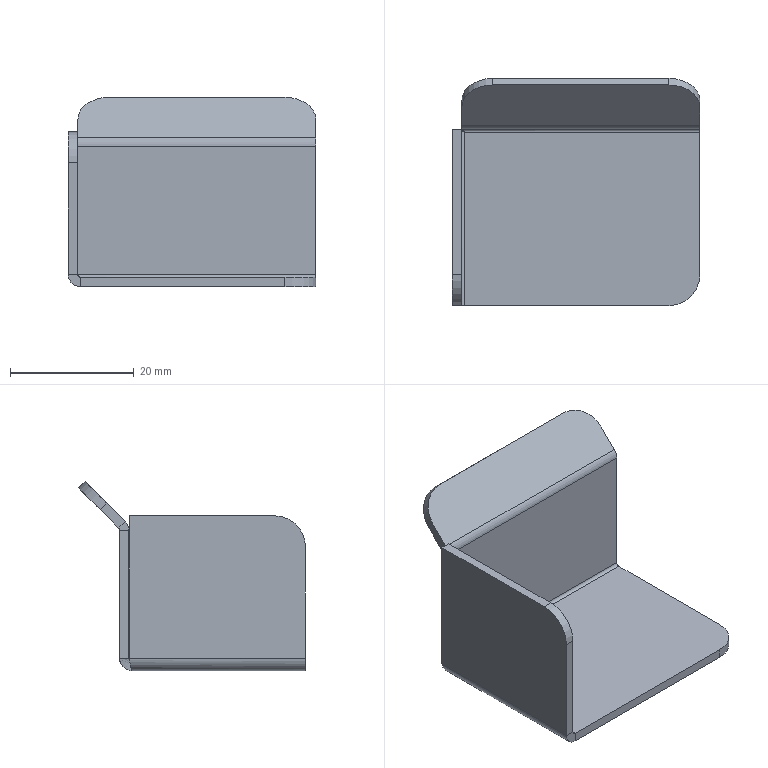Part | SolidWorks | features BaseBody 1 | 1 solid | 34 faces | box 40 x 36.632 x 30.571 mm | volume 4517 mm3 | plane 22 | cylinder 10 | spline 2 | commonest cylinder face diameters 10 x4 1 x3 4 x3
STEP:
#1=CARTESIAN_POINT('',(-13.429,20.571,29.071));
#2=VERTEX_POINT('',#1);
#3=CARTESIAN_POINT('',(-18.429,17.036,25.536));
#4=VERTEX_POINT('',#3);
#5=CARTESIAN_POINT('',(-13.429,17.036,25.536));
#6=DIRECTION('',(0.,-0.7071,0.7071));
#7=DIRECTION('',(0.,0.7071,0.7071));
#8=AXIS2_PLACEMENT_3D('',#5,#6,#7);
#9=CIRCLE('',#8,5.);
#10=EDGE_CURVE('',#2,#4,#9,.T.);
#11=ORIENTED_EDGE('',*,*,#10,.F.);
#12=CARTESIAN_POINT('',(-13.429,21.632,28.01));
#13=VERTEX_POINT('',#12);
#14=CARTESIAN_POINT('',(-13.429,20.571,29.071));
#15=DIRECTION('',(0.,-0.7071,0.7071));
#16=VECTOR('',#15,1000.);
#17=LINE('',#14,#16);
#18=EDGE_CURVE('',#13,#2,#17,.T.);
#19=ORIENTED_EDGE('',*,*,#18,.F.);
#20=CARTESIAN_POINT('',(-18.429,18.096,24.475));
#21=VERTEX_POINT('',#20);
#22=CARTESIAN_POINT('',(-13.429,18.096,24.475));
#23=DIRECTION('',(0.,0.7071,-0.7071));
#24=DIRECTION('',(0.,0.7071,0.7071));
#25=AXIS2_PLACEMENT_3D('',#22,#23,#24);
#26=CIRCLE('',#25,5.);
#27=EDGE_CURVE('',#21,#13,#26,.T.);
#28=ORIENTED_EDGE('',*,*,#27,.F.);
#29=CARTESIAN_POINT('',(-18.429,17.036,25.536));
#30=DIRECTION('',(0.,0.7071,-0.7071));
#31=VECTOR('',#30,1000.);
#32=LINE('',#29,#31);
#33=EDGE_CURVE('',#4,#21,#32,.T.);
#34=ORIENTED_EDGE('',*,*,#33,.F.);
#35=EDGE_LOOP('',(#11,#19,#28,#34));
#36=FACE_OUTER_BOUND('',#35,.T.);
#37=CARTESIAN_POINT('',(-13.429,17.036,25.536));
#38=DIRECTION('',(0.,0.7071,-0.7071));
#39=DIRECTION('',(0.,0.7071,0.7071));
#40=AXIS2_PLACEMENT_3D('',#37,#38,#39);
#41=CYLINDRICAL_SURFACE('',#40,5.);
#42=ADVANCED_FACE('',(#36),#41,.T.);
#43=CARTESIAN_POINT('',(20.,17.036,25.536));
#44=VERTEX_POINT('',#43);
#45=CARTESIAN_POINT('',(15.,20.571,29.071));
#46=VERTEX_POINT('',#45);
#47=CARTESIAN_POINT('',(15.,17.036,25.536));
#48=DIRECTION('',(0.,-0.7071,0.7071));
#49=DIRECTION('',(0.,0.7071,0.7071));
#50=AXIS2_PLACEMENT_3D('',#47,#48,#49);
#51=CIRCLE('',#50,5.);
#52=EDGE_CURVE('',#44,#46,#51,.T.);
#53=ORIENTED_EDGE('',*,*,#52,.F.);
#54=CARTESIAN_POINT('',(20.,18.096,24.475));
#55=VERTEX_POINT('',#54);
#56=CARTESIAN_POINT('',(20.,17.036,25.536));
#57=DIRECTION('',(0.,-0.7071,0.7071));
#58=VECTOR('',#57,1000.);
#59=LINE('',#56,#58);
#60=EDGE_CURVE('',#55,#44,#59,.T.);
#61=ORIENTED_EDGE('',*,*,#60,.F.);
#62=CARTESIAN_POINT('',(15.,21.632,28.01));
#63=VERTEX_POINT('',#62);
#64=CARTESIAN_POINT('',(15.,18.096,24.475));
#65=DIRECTION('',(0.,0.7071,-0.7071));
#66=DIRECTION('',(0.,0.7071,0.7071));
#67=AXIS2_PLACEMENT_3D('',#64,#65,#66);
#68=CIRCLE('',#67,5.);
#69=EDGE_CURVE('',#63,#55,#68,.T.);
#70=ORIENTED_EDGE('',*,*,#69,.F.);
#71=CARTESIAN_POINT('',(15.,20.571,29.071));
#72=DIRECTION('',(0.,0.7071,-0.7071));
#73=VECTOR('',#72,1000.);
#74=LINE('',#71,#73);
#75=EDGE_CURVE('',#46,#63,#74,.T.);
#76=ORIENTED_EDGE('',*,*,#75,.F.);
#77=EDGE_LOOP('',(#53,#61,#70,#76));
#78=FACE_OUTER_BOUND('',#77,.T.);
#79=CARTESIAN_POINT('',(15.,17.036,25.536));
#80=DIRECTION('',(0.,0.7071,-0.7071));
#81=DIRECTION('',(0.,0.7071,0.7071));
#82=AXIS2_PLACEMENT_3D('',#79,#80,#81);
#83=CYLINDRICAL_SURFACE('',#82,5.);
#84=ADVANCED_FACE('',(#78),#83,.T.);
#85=CARTESIAN_POINT('',(-20.,-15.,18.5));
#86=VERTEX_POINT('',#85);
#87=CARTESIAN_POINT('',(-20.,-10.,23.5));
#88=VERTEX_POINT('',#87);
#89=CARTESIAN_POINT('',(-20.,-10.,18.5));
#90=DIRECTION('',(-1.,0.,0.));
#91=DIRECTION('',(0.,0.,-1.));
#92=AXIS2_PLACEMENT_3D('',#89,#90,#91);
#93=CIRCLE('',#92,5.);
#94=EDGE_CURVE('',#86,#88,#93,.T.);
#95=ORIENTED_EDGE('',*,*,#94,.F.);
#96=CARTESIAN_POINT('',(-18.5,-15.,18.5));
#97=VERTEX_POINT('',#96);
#98=CARTESIAN_POINT('',(-20.,-15.,18.5));
#99=DIRECTION('',(-1.,0.,0.));
#100=VECTOR('',#99,1000.);
#101=LINE('',#98,#100);
#102=EDGE_CURVE('',#97,#86,#101,.T.);
#103=ORIENTED_EDGE('',*,*,#102,.F.);
#104=CARTESIAN_POINT('',(-18.5,-10.,23.5));
#105=VERTEX_POINT('',#104);
#106=CARTESIAN_POINT('',(-18.5,-10.,18.5));
#107=DIRECTION('',(1.,0.,0.));
#108=DIRECTION('',(0.,0.,-1.));
#109=AXIS2_PLACEMENT_3D('',#106,#107,#108);
#110=CIRCLE('',#109,5.);
#111=EDGE_CURVE('',#105,#97,#110,.T.);
#112=ORIENTED_EDGE('',*,*,#111,.F.);
#113=CARTESIAN_POINT('',(-20.,-10.,23.5));
#114=DIRECTION('',(1.,0.,0.));
#115=VECTOR('',#114,1000.);
#116=LINE('',#113,#115);
#117=EDGE_CURVE('',#88,#105,#116,.T.);
#118=ORIENTED_EDGE('',*,*,#117,.F.);
#119=EDGE_LOOP('',(#95,#103,#112,#118));
#120=FACE_OUTER_BOUND('',#119,.T.);
#121=CARTESIAN_POINT('',(-20.,-10.,18.5));
#122=DIRECTION('',(1.,0.,0.));
#123=DIRECTION('',(0.,0.,-1.));
#124=AXIS2_PLACEMENT_3D('',#121,#122,#123);
#125=CYLINDRICAL_SURFACE('',#124,5.);
#126=ADVANCED_FACE('',(#120),#125,.T.);
#127=CARTESIAN_POINT('',(20.,-10.,-1.5));
#128=VERTEX_POINT('',#127);
#129=CARTESIAN_POINT('',(15.,-15.,-1.5));
#130=VERTEX_POINT('',#129);
#131=CARTESIAN_POINT('',(15.,-10.,-1.5));
#132=DIRECTION('',(0.,0.,-1.));
#133=DIRECTION('',(-1.,0.,0.));
#134=AXIS2_PLACEMENT_3D('',#131,#132,#133);
#135=CIRCLE('',#134,5.);
#136=EDGE_CURVE('',#128,#130,#135,.T.);
#137=ORIENTED_EDGE('',*,*,#136,.F.);
#138=CARTESIAN_POINT('',(20.,-10.,0.));
#139=VERTEX_POINT('',#138);
#140=CARTESIAN_POINT('',(20.,-10.,-1.5));
#141=DIRECTION('',(0.,0.,-1.));
#142=VECTOR('',#141,1000.);
#143=LINE('',#140,#142);
#144=EDGE_CURVE('',#139,#128,#143,.T.);
#145=ORIENTED_EDGE('',*,*,#144,.F.);
#146=CARTESIAN_POINT('',(15.,-15.,0.));
#147=VERTEX_POINT('',#146);
#148=CARTESIAN_POINT('',(15.,-10.,0.));
#149=DIRECTION('',(0.,0.,1.));
#150=DIRECTION('',(-1.,0.,0.));
#151=AXIS2_PLACEMENT_3D('',#148,#149,#150);
#152=CIRCLE('',#151,5.);
#153=EDGE_CURVE('',#147,#139,#152,.T.);
#154=ORIENTED_EDGE('',*,*,#153,.F.);
#155=CARTESIAN_POINT('',(15.,-15.,-1.5));
#156=DIRECTION('',(0.,0.,1.));
#157=VECTOR('',#156,1000.);
#158=LINE('',#155,#157);
#159=EDGE_CURVE('',#130,#147,#158,.T.);
#160=ORIENTED_EDGE('',*,*,#159,.F.);
#161=EDGE_LOOP('',(#137,#145,#154,#160));
#162=FACE_OUTER_BOUND('',#161,.T.);
#163=CARTESIAN_POINT('',(15.,-10.,-1.5));
#164=DIRECTION('',(0.,0.,1.));
#165=DIRECTION('',(1.,0.,0.));
#166=AXIS2_PLACEMENT_3D('',#163,#164,#165);
#167=CYLINDRICAL_SURFACE('',#166,5.);
#168=ADVANCED_FACE('',(#162),#167,.T.);
#169=CARTESIAN_POINT('',(0.,20.571,29.071));
#170=DIRECTION('',(-1.,0.,0.));
#171=VECTOR('',#170,1000.);
#172=LINE('',#169,#171);
#173=EDGE_CURVE('',#46,#2,#172,.T.);
#174=ORIENTED_EDGE('',*,*,#173,.F.);
#175=ORIENTED_EDGE('',*,*,#75,.T.);
#176=CARTESIAN_POINT('',(-18.429,21.632,28.01));
#177=DIRECTION('',(-1.,0.,0.));
#178=VECTOR('',#177,1000.);
#179=LINE('',#176,#178);
#180=EDGE_CURVE('',#63,#13,#179,.T.);
#181=ORIENTED_EDGE('',*,*,#180,.T.);
#182=ORIENTED_EDGE('',*,*,#18,.T.);
#183=EDGE_LOOP('',(#174,#175,#181,#182));
#184=FACE_OUTER_BOUND('',#183,.T.);
#185=CARTESIAN_POINT('',(-18.429,20.571,29.071));
#186=DIRECTION('',(0.,-0.7071,-0.7071));
#187=DIRECTION('',(0.,-0.7071,0.7071));
#188=AXIS2_PLACEMENT_3D('',#185,#186,#187);
#189=PLANE('',#188);
#190=ADVANCED_FACE('',(#184),#189,.F.);
#191=ORIENTED_EDGE('',*,*,#180,.F.);
#192=ORIENTED_EDGE('',*,*,#69,.T.);
#193=CARTESIAN_POINT('',(20.,15.146,21.525));
#194=VERTEX_POINT('',#193);
#195=CARTESIAN_POINT('',(20.,21.632,28.01));
#196=DIRECTION('',(0.,0.7071,0.7071));
#197=VECTOR('',#196,1000.);
#198=LINE('',#195,#197);
#199=EDGE_CURVE('',#194,#55,#198,.T.);
#200=ORIENTED_EDGE('',*,*,#199,.F.);
#201=CARTESIAN_POINT('',(-18.429,15.146,21.525));
#202=VERTEX_POINT('',#201);
#203=CARTESIAN_POINT('',(-18.429,15.146,21.525));
#204=DIRECTION('',(1.,0.,0.));
#205=VECTOR('',#204,1000.);
#206=LINE('',#203,#205);
#207=EDGE_CURVE('',#202,#194,#206,.T.);
#208=ORIENTED_EDGE('',*,*,#207,.F.);
#209=CARTESIAN_POINT('',(-18.429,15.,21.379));
#210=DIRECTION('',(0.,-0.7071,-0.7071));
#211=VECTOR('',#210,1000.);
#212=LINE('',#209,#211);
#213=EDGE_CURVE('',#21,#202,#212,.T.);
#214=ORIENTED_EDGE('',*,*,#213,.F.);
#215=ORIENTED_EDGE('',*,*,#27,.T.);
#216=EDGE_LOOP('',(#191,#192,#200,#208,#214,#215));
#217=FACE_OUTER_BOUND('',#216,.T.);
#218=CARTESIAN_POINT('',(0.,-4.25,2.129));
#219=DIRECTION('',(0.,0.7071,-0.7071));
#220=DIRECTION('',(-1.,0.,0.));
#221=AXIS2_PLACEMENT_3D('',#218,#219,#220);
#222=PLANE('',#221);
#223=ADVANCED_FACE('',(#217),#222,.T.);
#224=CARTESIAN_POINT('',(20.,14.086,22.586));
#225=VERTEX_POINT('',#224);
#226=CARTESIAN_POINT('',(20.,-5.311,3.189));
#227=DIRECTION('',(0.,0.7071,0.7071));
#228=VECTOR('',#227,1000.);
#229=LINE('',#226,#228);
#230=EDGE_CURVE('',#225,#44,#229,.T.);
#231=ORIENTED_EDGE('',*,*,#230,.T.);
#232=ORIENTED_EDGE('',*,*,#52,.T.);
#233=ORIENTED_EDGE('',*,*,#173,.T.);
#234=ORIENTED_EDGE('',*,*,#10,.T.);
#235=CARTESIAN_POINT('',(-18.429,14.086,22.586));
#236=VERTEX_POINT('',#235);
#237=CARTESIAN_POINT('',(-18.429,-5.311,3.189));
#238=DIRECTION('',(0.,-0.7071,-0.7071));
#239=VECTOR('',#238,1000.);
#240=LINE('',#237,#239);
#241=EDGE_CURVE('',#4,#236,#240,.T.);
#242=ORIENTED_EDGE('',*,*,#241,.T.);
#243=CARTESIAN_POINT('',(-18.429,14.086,22.586));
#244=DIRECTION('',(-1.,0.,0.));
#245=VECTOR('',#244,1000.);
#246=LINE('',#243,#245);
#247=EDGE_CURVE('',#225,#236,#246,.T.);
#248=ORIENTED_EDGE('',*,*,#247,.F.);
#249=EDGE_LOOP('',(#231,#232,#233,#234,#242,#248));
#250=FACE_OUTER_BOUND('',#249,.T.);
#251=CARTESIAN_POINT('',(0.,-5.311,3.189));
#252=DIRECTION('',(0.,0.7071,-0.7071));
#253=DIRECTION('',(-1.,0.,0.));
#254=AXIS2_PLACEMENT_3D('',#251,#252,#253);
#255=PLANE('',#254);
#256=ADVANCED_FACE('',(#250),#255,.F.);
#257=ORIENTED_EDGE('',*,*,#199,.T.);
#258=ORIENTED_EDGE('',*,*,#60,.T.);
#259=ORIENTED_EDGE('',*,*,#230,.F.);
#260=CARTESIAN_POINT('',(20.,15.146,21.525));
#261=DIRECTION('',(0.,-0.7071,0.7071));
#262=VECTOR('',#261,1000.);
#263=LINE('',#260,#262);
#264=EDGE_CURVE('',#194,#225,#263,.T.);
#265=ORIENTED_EDGE('',*,*,#264,.F.);
#266=EDGE_LOOP('',(#257,#258,#259,#265));
#267=FACE_OUTER_BOUND('',#266,.T.);
#268=CARTESIAN_POINT('',(20.,20.571,29.071));
#269=DIRECTION('',(-1.,0.,0.));
#270=DIRECTION('',(0.,1.,0.));
#271=AXIS2_PLACEMENT_3D('',#268,#269,#270);
#272=PLANE('',#271);
#273=ADVANCED_FACE('',(#267),#272,.F.);
#274=ORIENTED_EDGE('',*,*,#241,.F.);
#275=ORIENTED_EDGE('',*,*,#33,.T.);
#276=ORIENTED_EDGE('',*,*,#213,.T.);
#277=CARTESIAN_POINT('',(-18.429,14.086,22.586));
#278=DIRECTION('',(0.,-0.7071,0.7071));
#279=VECTOR('',#278,1000.);
#280=LINE('',#277,#279);
#281=EDGE_CURVE('',#202,#236,#280,.T.);
#282=ORIENTED_EDGE('',*,*,#281,.T.);
#283=EDGE_LOOP('',(#274,#275,#276,#282));
#284=FACE_OUTER_BOUND('',#283,.T.);
#285=CARTESIAN_POINT('',(-18.429,13.939,22.439));
#286=DIRECTION('',(1.,0.,0.));
#287=DIRECTION('',(0.,1.,0.));
#288=AXIS2_PLACEMENT_3D('',#285,#286,#287);
#289=PLANE('',#288);
#290=ADVANCED_FACE('',(#284),#289,.F.);
#291=CARTESIAN_POINT('',(20.,15.,21.172));
#292=VERTEX_POINT('',#291);
#293=CARTESIAN_POINT('',(-18.429,15.,21.172));
#294=VERTEX_POINT('',#293);
#295=CARTESIAN_POINT('',(20.,15.,21.172));
#296=DIRECTION('',(-1.,0.,0.));
#297=VECTOR('',#296,1000.);
#298=LINE('',#295,#297);
#299=EDGE_CURVE('',#292,#294,#298,.T.);
#300=ORIENTED_EDGE('',*,*,#299,.T.);
#301=CARTESIAN_POINT('',(-18.429,15.5,21.172));
#302=DIRECTION('',(-1.,0.,0.));
#303=DIRECTION('',(0.,0.,-1.));
#304=AXIS2_PLACEMENT_3D('',#301,#302,#303);
#305=CIRCLE('',#304,0.5);
#306=EDGE_CURVE('',#294,#202,#305,.T.);
#307=ORIENTED_EDGE('',*,*,#306,.T.);
#308=ORIENTED_EDGE('',*,*,#207,.T.);
#309=CARTESIAN_POINT('',(20.,15.5,21.172));
#310=DIRECTION('',(1.,0.,0.));
#311=DIRECTION('',(0.,0.,-1.));
#312=AXIS2_PLACEMENT_3D('',#309,#310,#311);
#313=CIRCLE('',#312,0.5);
#314=EDGE_CURVE('',#194,#292,#313,.T.);
#315=ORIENTED_EDGE('',*,*,#314,.T.);
#316=EDGE_LOOP('',(#300,#307,#308,#315));
#317=FACE_OUTER_BOUND('',#316,.T.);
#318=CARTESIAN_POINT('',(20.,15.5,21.172));
#319=DIRECTION('',(1.,0.,0.));
#320=DIRECTION('',(0.,-0.7071,0.7071));
#321=AXIS2_PLACEMENT_3D('',#318,#319,#320);
#322=CYLINDRICAL_SURFACE('',#321,0.5);
#323=ADVANCED_FACE('',(#317),#322,.F.);
#324=CARTESIAN_POINT('',(20.,13.5,21.172));
#325=VERTEX_POINT('',#324);
#326=CARTESIAN_POINT('',(-18.429,13.5,21.172));
#327=VERTEX_POINT('',#326);
#328=CARTESIAN_POINT('',(20.,13.5,21.172));
#329=DIRECTION('',(-1.,0.,0.));
#330=VECTOR('',#329,1000.);
#331=LINE('',#328,#330);
#332=EDGE_CURVE('',#325,#327,#331,.T.);
#333=ORIENTED_EDGE('',*,*,#332,.F.);
#334=CARTESIAN_POINT('',(20.,15.5,21.172));
#335=DIRECTION('',(1.,0.,0.));
#336=DIRECTION('',(0.,0.,-1.));
#337=AXIS2_PLACEMENT_3D('',#334,#335,#336);
#338=CIRCLE('',#337,2.);
#339=EDGE_CURVE('',#225,#325,#338,.T.);
#340=ORIENTED_EDGE('',*,*,#339,.F.);
#341=ORIENTED_EDGE('',*,*,#247,.T.);
#342=CARTESIAN_POINT('',(-18.429,15.5,21.172));
#343=DIRECTION('',(-1.,0.,0.));
#344=DIRECTION('',(0.,0.,-1.));
#345=AXIS2_PLACEMENT_3D('',#342,#343,#344);
#346=CIRCLE('',#345,2.);
#347=EDGE_CURVE('',#327,#236,#346,.T.);
#348=ORIENTED_EDGE('',*,*,#347,.F.);
#349=EDGE_LOOP('',(#333,#340,#341,#348));
#350=FACE_OUTER_BOUND('',#349,.T.);
#351=CARTESIAN_POINT('',(20.,15.5,21.172));
#352=DIRECTION('',(1.,0.,0.));
#353=DIRECTION('',(0.,-0.7071,0.7071));
#354=AXIS2_PLACEMENT_3D('',#351,#352,#353);
#355=CYLINDRICAL_SURFACE('',#354,2.);
#356=ADVANCED_FACE('',(#350),#355,.T.);
#357=ORIENTED_EDGE('',*,*,#314,.F.);
#358=ORIENTED_EDGE('',*,*,#264,.T.);
#359=ORIENTED_EDGE('',*,*,#339,.T.);
#360=CARTESIAN_POINT('',(20.,15.,21.172));
#361=DIRECTION('',(0.,-1.,0.));
#362=VECTOR('',#361,1000.);
#363=LINE('',#360,#362);
#364=EDGE_CURVE('',#292,#325,#363,.T.);
#365=ORIENTED_EDGE('',*,*,#364,.F.);
#366=EDGE_LOOP('',(#357,#358,#359,#365));
#367=FACE_OUTER_BOUND('',#366,.T.);
#368=CARTESIAN_POINT('',(20.,15.5,21.172));
#369=DIRECTION('',(-1.,0.,0.));
#370=DIRECTION('',(0.,0.,1.));
#371=AXIS2_PLACEMENT_3D('',#368,#369,#370);
#372=PLANE('',#371);
#373=ADVANCED_FACE('',(#367),#372,.F.);
#374=ORIENTED_EDGE('',*,*,#281,.F.);
#375=ORIENTED_EDGE('',*,*,#306,.F.);
#376=CARTESIAN_POINT('',(-18.429,15.,21.172));
#377=DIRECTION('',(0.,-1.,0.));
#378=VECTOR('',#377,1000.);
#379=LINE('',#376,#378);
#380=EDGE_CURVE('',#294,#327,#379,.T.);
#381=ORIENTED_EDGE('',*,*,#380,.T.);
#382=ORIENTED_EDGE('',*,*,#347,.T.);
#383=EDGE_LOOP('',(#374,#375,#381,#382));
#384=FACE_OUTER_BOUND('',#383,.T.);
#385=CARTESIAN_POINT('',(-18.429,15.5,21.172));
#386=DIRECTION('',(-1.,0.,0.));
#387=DIRECTION('',(0.,0.,1.));
#388=AXIS2_PLACEMENT_3D('',#385,#386,#387);
#389=PLANE('',#388);
#390=ADVANCED_FACE('',(#384),#389,.T.);
#391=CARTESIAN_POINT('',(-18.5,-15.,0.5));
#392=VERTEX_POINT('',#391);
#393=CARTESIAN_POINT('',(-18.5,-15.,23.5));
#394=DIRECTION('',(0.,0.,1.));
#395=VECTOR('',#394,1000.);
#396=LINE('',#393,#395);
#397=EDGE_CURVE('',#392,#97,#396,.T.);
#398=ORIENTED_EDGE('',*,*,#397,.T.);
#399=ORIENTED_EDGE('',*,*,#102,.T.);
#400=CARTESIAN_POINT('',(-20.,-15.,0.5));
#401=VERTEX_POINT('',#400);
#402=CARTESIAN_POINT('',(-20.,-15.,0.));
#403=DIRECTION('',(0.,0.,1.));
#404=VECTOR('',#403,1000.);
#405=LINE('',#402,#404);
#406=EDGE_CURVE('',#401,#86,#405,.T.);
#407=ORIENTED_EDGE('',*,*,#406,.F.);
#408=CARTESIAN_POINT('',(-18.5,-15.,0.5));
#409=DIRECTION('',(-1.,0.,0.));
#410=VECTOR('',#409,1000.);
#411=LINE('',#408,#410);
#412=EDGE_CURVE('',#392,#401,#411,.T.);
#413=ORIENTED_EDGE('',*,*,#412,.F.);
#414=EDGE_LOOP('',(#398,#399,#407,#413));
#415=FACE_OUTER_BOUND('',#414,.T.);
#416=CARTESIAN_POINT('',(-20.,-15.,23.5));
#417=DIRECTION('',(0.,1.,0.));
#418=DIRECTION('',(0.,0.,-1.));
#419=AXIS2_PLACEMENT_3D('',#416,#417,#418);
#420=PLANE('',#419);
#421=ADVANCED_FACE('',(#415),#420,.F.);
#422=CARTESIAN_POINT('',(-20.,13.429,23.5));
#423=VERTEX_POINT('',#422);
#424=CARTESIAN_POINT('',(-20.,0.,23.5));
#425=DIRECTION('',(0.,1.,0.));
#426=VECTOR('',#425,1000.);
#427=LINE('',#424,#426);
#428=EDGE_CURVE('',#88,#423,#427,.T.);
#429=ORIENTED_EDGE('',*,*,#428,.F.);
#430=ORIENTED_EDGE('',*,*,#117,.T.);
#431=CARTESIAN_POINT('',(-18.5,13.429,23.5));
#432=VERTEX_POINT('',#431);
#433=CARTESIAN_POINT('',(-18.5,15.,23.5));
#434=DIRECTION('',(0.,1.,0.));
#435=VECTOR('',#434,1000.);
#436=LINE('',#433,#435);
#437=EDGE_CURVE('',#105,#432,#436,.T.);
#438=ORIENTED_EDGE('',*,*,#437,.T.);
#439=CARTESIAN_POINT('',(-18.5,13.429,23.5));
#440=DIRECTION('',(1.,0.,0.));
#441=VECTOR('',#440,1000.);
#442=LINE('',#439,#441);
#443=EDGE_CURVE('',#423,#432,#442,.T.);
#444=ORIENTED_EDGE('',*,*,#443,.F.);
#445=EDGE_LOOP('',(#429,#430,#438,#444));
#446=FACE_OUTER_BOUND('',#445,.T.);
#447=CARTESIAN_POINT('',(-20.,15.,23.5));
#448=DIRECTION('',(0.,0.,-1.));
#449=DIRECTION('',(0.,-1.,0.));
#450=AXIS2_PLACEMENT_3D('',#447,#448,#449);
#451=PLANE('',#450);
#452=ADVANCED_FACE('',(#446),#451,.F.);
#453=ORIENTED_EDGE('',*,*,#437,.F.);
#454=ORIENTED_EDGE('',*,*,#111,.T.);
#455=ORIENTED_EDGE('',*,*,#397,.F.);
#456=CARTESIAN_POINT('',(-18.5,13.429,0.5));
#457=VERTEX_POINT('',#456);
#458=CARTESIAN_POINT('',(-18.5,15.,0.5));
#459=DIRECTION('',(0.,-1.,0.));
#460=VECTOR('',#459,1000.);
#461=LINE('',#458,#460);
#462=EDGE_CURVE('',#457,#392,#461,.T.);
#463=ORIENTED_EDGE('',*,*,#462,.F.);
#464=CARTESIAN_POINT('',(-18.5,13.429,0.));
#465=DIRECTION('',(0.,0.,1.));
#466=VECTOR('',#465,1000.);
#467=LINE('',#464,#466);
#468=EDGE_CURVE('',#457,#432,#467,.T.);
#469=ORIENTED_EDGE('',*,*,#468,.T.);
#470=EDGE_LOOP('',(#453,#454,#455,#463,#469));
#471=FACE_OUTER_BOUND('',#470,.T.);
#472=CARTESIAN_POINT('',(-18.5,0.,0.));
#473=DIRECTION('',(1.,0.,0.));
#474=DIRECTION('',(0.,0.,1.));
#475=AXIS2_PLACEMENT_3D('',#472,#473,#474);
#476=PLANE('',#475);
#477=ADVANCED_FACE('',(#471),#476,.T.);
#478=ORIENTED_EDGE('',*,*,#406,.T.);
#479=ORIENTED_EDGE('',*,*,#94,.T.);
#480=ORIENTED_EDGE('',*,*,#428,.T.);
#481=CARTESIAN_POINT('',(-20.,13.429,0.5));
#482=VERTEX_POINT('',#481);
#483=CARTESIAN_POINT('',(-20.,13.429,0.));
#484=DIRECTION('',(0.,0.,1.));
#485=VECTOR('',#484,1000.);
#486=LINE('',#483,#485);
#487=EDGE_CURVE('',#482,#423,#486,.T.);
#488=ORIENTED_EDGE('',*,*,#487,.F.);
#489=CARTESIAN_POINT('',(-20.,15.,0.5));
#490=DIRECTION('',(0.,1.,0.));
#491=VECTOR('',#490,1000.);
#492=LINE('',#489,#491);
#493=EDGE_CURVE('',#401,#482,#492,.T.);
#494=ORIENTED_EDGE('',*,*,#493,.F.);
#495=EDGE_LOOP('',(#478,#479,#480,#488,#494));
#496=FACE_OUTER_BOUND('',#495,.T.);
#497=CARTESIAN_POINT('',(-20.,0.,0.));
#498=DIRECTION('',(1.,0.,0.));
#499=DIRECTION('',(0.,0.,1.));
#500=AXIS2_PLACEMENT_3D('',#497,#498,#499);
#501=PLANE('',#500);
#502=ADVANCED_FACE('',(#496),#501,.F.);
#503=ORIENTED_EDGE('',*,*,#487,.T.);
#504=ORIENTED_EDGE('',*,*,#443,.T.);
#505=ORIENTED_EDGE('',*,*,#468,.F.);
#506=CARTESIAN_POINT('',(-18.5,13.429,0.5));
#507=DIRECTION('',(1.,0.,0.));
#508=VECTOR('',#507,1000.);
#509=LINE('',#506,#508);
#510=EDGE_CURVE('',#482,#457,#509,.T.);
#511=ORIENTED_EDGE('',*,*,#510,.F.);
#512=EDGE_LOOP('',(#503,#504,#505,#511));
#513=FACE_OUTER_BOUND('',#512,.T.);
#514=CARTESIAN_POINT('',(-18.5,13.429,0.));
#515=DIRECTION('',(0.,1.,0.));
#516=DIRECTION('',(1.,0.,0.));
#517=AXIS2_PLACEMENT_3D('',#514,#515,#516);
#518=PLANE('',#517);
#519=ADVANCED_FACE('',(#513),#518,.T.);
#520=CARTESIAN_POINT('',(-18.,-15.,0.));
#521=VERTEX_POINT('',#520);
#522=CARTESIAN_POINT('',(-18.,13.,0.));
#523=VERTEX_POINT('',#522);
#524=CARTESIAN_POINT('',(-18.,-15.,0.));
#525=DIRECTION('',(0.,1.,0.));
#526=VECTOR('',#525,1000.);
#527=LINE('',#524,#526);
#528=EDGE_CURVE('',#521,#523,#527,.T.);
#529=ORIENTED_EDGE('',*,*,#528,.T.);
#530=CARTESIAN_POINT('',(-18.,13.,0.));
#531=CARTESIAN_POINT('',(-18.131,13.072,0.));
#532=CARTESIAN_POINT('',(-18.261,13.143,0.05389));
#533=CARTESIAN_POINT('',(-18.446,13.286,0.239));
#534=CARTESIAN_POINT('',(-18.5,13.358,0.3691));
#535=CARTESIAN_POINT('',(-18.5,13.429,0.5));
#536=B_SPLINE_CURVE_WITH_KNOTS('',3,(#530,#531,#532,#533,#534,#535),.UNSPECIFIED.,.F.,.F.,(4,2,4),(0.,0.5,1.),.UNSPECIFIED.);
#537=EDGE_CURVE('',#523,#457,#536,.T.);
#538=ORIENTED_EDGE('',*,*,#537,.T.);
#539=ORIENTED_EDGE('',*,*,#462,.T.);
#540=CARTESIAN_POINT('',(-18.,-15.,0.5));
#541=DIRECTION('',(0.,-1.,0.));
#542=DIRECTION('',(0.,0.,-1.));
#543=AXIS2_PLACEMENT_3D('',#540,#541,#542);
#544=CIRCLE('',#543,0.5);
#545=EDGE_CURVE('',#392,#521,#544,.T.);
#546=ORIENTED_EDGE('',*,*,#545,.T.);
#547=EDGE_LOOP('',(#529,#538,#539,#546));
#548=FACE_OUTER_BOUND('',#547,.T.);
#549=CARTESIAN_POINT('',(-18.,-15.,0.5));
#550=DIRECTION('',(0.,-1.,0.));
#551=DIRECTION('',(-1.,0.,0.));
#552=AXIS2_PLACEMENT_3D('',#549,#550,#551);
#553=CYLINDRICAL_SURFACE('',#552,0.5);
#554=ADVANCED_FACE('',(#548),#553,.F.);
#555=CARTESIAN_POINT('',(-18.,-15.,-1.5));
#556=VERTEX_POINT('',#555);
#557=CARTESIAN_POINT('',(-18.,13.,-1.5));
#558=VERTEX_POINT('',#557);
#559=CARTESIAN_POINT('',(-18.,-15.,-1.5));
#560=DIRECTION('',(0.,1.,0.));
#561=VECTOR('',#560,1000.);
#562=LINE('',#559,#561);
#563=EDGE_CURVE('',#556,#558,#562,.T.);
#564=ORIENTED_EDGE('',*,*,#563,.F.);
#565=CARTESIAN_POINT('',(-18.,-15.,0.5));
#566=DIRECTION('',(0.,-1.,0.));
#567=DIRECTION('',(0.,0.,-1.));
#568=AXIS2_PLACEMENT_3D('',#565,#566,#567);
#569=CIRCLE('',#568,2.);
#570=EDGE_CURVE('',#401,#556,#569,.T.);
#571=ORIENTED_EDGE('',*,*,#570,.F.);
#572=ORIENTED_EDGE('',*,*,#493,.T.);
#573=CARTESIAN_POINT('',(-18.,13.,-1.5));
#574=CARTESIAN_POINT('',(-18.262,13.036,-1.5));
#575=CARTESIAN_POINT('',(-18.523,13.072,-1.448));
#576=CARTESIAN_POINT('',(-19.007,13.143,-1.248));
#577=CARTESIAN_POINT('',(-19.229,13.179,-1.099));
#578=CARTESIAN_POINT('',(-19.599,13.25,-0.7291));
#579=CARTESIAN_POINT('',(-19.748,13.286,-0.5072));
#580=CARTESIAN_POINT('',(-19.948,13.358,-0.0235));
#581=CARTESIAN_POINT('',(-20.,13.394,0.2382));
#582=CARTESIAN_POINT('',(-20.,13.429,0.5));
#583=B_SPLINE_CURVE_WITH_KNOTS('',3,(#573,#574,#575,#576,#577,#578,#579,#580,#581,#582),.UNSPECIFIED.,.F.,.F.,(4,2,2,2,4),(0.,0.25,0.5,0.75,1.),.UNSPECIFIED.);
#584=EDGE_CURVE('',#558,#482,#583,.T.);
#585=ORIENTED_EDGE('',*,*,#584,.F.);
#586=EDGE_LOOP('',(#564,#571,#572,#585));
#587=FACE_OUTER_BOUND('',#586,.T.);
#588=CARTESIAN_POINT('',(-18.,-15.,0.5));
#589=DIRECTION('',(0.,-1.,0.));
#590=DIRECTION('',(-1.,0.,0.));
#591=AXIS2_PLACEMENT_3D('',#588,#589,#590);
#592=CYLINDRICAL_SURFACE('',#591,2.);
#593=ADVANCED_FACE('',(#587),#592,.T.);
#594=ORIENTED_EDGE('',*,*,#545,.F.);
#595=ORIENTED_EDGE('',*,*,#412,.T.);
#596=ORIENTED_EDGE('',*,*,#570,.T.);
#597=CARTESIAN_POINT('',(-18.,-15.,0.));
#598=DIRECTION('',(0.,0.,-1.));
#599=VECTOR('',#598,1000.);
#600=LINE('',#597,#599);
#601=EDGE_CURVE('',#521,#556,#600,.T.);
#602=ORIENTED_EDGE('',*,*,#601,.F.);
#603=EDGE_LOOP('',(#594,#595,#596,#602));
#604=FACE_OUTER_BOUND('',#603,.T.);
#605=CARTESIAN_POINT('',(-18.,-15.,0.5));
#606=DIRECTION('',(0.,1.,0.));
#607=DIRECTION('',(1.,0.,0.));
#608=AXIS2_PLACEMENT_3D('',#605,#606,#607);
#609=PLANE('',#608);
#610=ADVANCED_FACE('',(#604),#609,.F.);
#611=ORIENTED_EDGE('',*,*,#510,.T.);
#612=ORIENTED_EDGE('',*,*,#537,.F.);
#613=CARTESIAN_POINT('',(-18.,13.,0.));
#614=DIRECTION('',(0.,0.,-1.));
#615=VECTOR('',#614,1000.);
#616=LINE('',#613,#615);
#617=EDGE_CURVE('',#523,#558,#616,.T.);
#618=ORIENTED_EDGE('',*,*,#617,.T.);
#619=ORIENTED_EDGE('',*,*,#584,.T.);
#620=EDGE_LOOP('',(#611,#612,#618,#619));
#621=FACE_OUTER_BOUND('',#620,.T.);
#622=CARTESIAN_POINT('',(-18.,13.,-1.515));
#623=CARTESIAN_POINT('',(-18.264,13.036,-1.515));
#624=CARTESIAN_POINT('',(-18.527,13.072,-1.463));
#625=CARTESIAN_POINT('',(-19.015,13.143,-1.261));
#626=CARTESIAN_POINT('',(-19.238,13.179,-1.111));
#627=CARTESIAN_POINT('',(-19.611,13.25,-0.7383));
#628=CARTESIAN_POINT('',(-19.761,13.286,-0.5148));
#629=CARTESIAN_POINT('',(-19.963,13.358,-0.02742));
#630=CARTESIAN_POINT('',(-20.015,13.394,0.2362));
#631=CARTESIAN_POINT('',(-20.015,13.429,0.5));
#632=CARTESIAN_POINT('',(-18.,13.,-1.5));
#633=CARTESIAN_POINT('',(-18.262,13.036,-1.5));
#634=CARTESIAN_POINT('',(-18.523,13.072,-1.448));
#635=CARTESIAN_POINT('',(-19.007,13.143,-1.248));
#636=CARTESIAN_POINT('',(-19.229,13.179,-1.099));
#637=CARTESIAN_POINT('',(-19.599,13.25,-0.7291));
#638=CARTESIAN_POINT('',(-19.748,13.286,-0.5072));
#639=CARTESIAN_POINT('',(-19.948,13.358,-0.0235));
#640=CARTESIAN_POINT('',(-20.,13.394,0.2382));
#641=CARTESIAN_POINT('',(-20.,13.429,0.5));
#642=CARTESIAN_POINT('',(-18.,13.,0.));
#643=CARTESIAN_POINT('',(-18.065,13.036,0.));
#644=CARTESIAN_POINT('',(-18.131,13.072,0.01301));
#645=CARTESIAN_POINT('',(-18.252,13.143,0.06311));
#646=CARTESIAN_POINT('',(-18.307,13.179,0.1002));
#647=CARTESIAN_POINT('',(-18.4,13.25,0.1927));
#648=CARTESIAN_POINT('',(-18.437,13.286,0.2482));
#649=CARTESIAN_POINT('',(-18.487,13.358,0.3691));
#650=CARTESIAN_POINT('',(-18.5,13.394,0.4345));
#651=CARTESIAN_POINT('',(-18.5,13.429,0.5));
#652=CARTESIAN_POINT('',(-18.,13.,0.01515));
#653=CARTESIAN_POINT('',(-18.063,13.036,0.01515));
#654=CARTESIAN_POINT('',(-18.127,13.072,0.02777));
#655=CARTESIAN_POINT('',(-18.244,13.143,0.07634));
#656=CARTESIAN_POINT('',(-18.298,13.179,0.1123));
#657=CARTESIAN_POINT('',(-18.388,13.25,0.202));
#658=CARTESIAN_POINT('',(-18.424,13.286,0.2558));
#659=CARTESIAN_POINT('',(-18.472,13.358,0.3731));
#660=CARTESIAN_POINT('',(-18.485,13.394,0.4365));
#661=CARTESIAN_POINT('',(-18.485,13.429,0.5));
#662=B_SPLINE_SURFACE_WITH_KNOTS('',1,3,((#622,#623,#624,#625,#626,#627,#628,#629,#630,#631),(#632,#633,#634,#635,#636,#637,#638,#639,#640,#641),(#642,#643,#644,#645,#646,#647,#648,#649,#650,#651),(#652,#653,#654,#655,#656,#657,#658,#659,#660,#661)),.UNSPECIFIED.,.F.,.F.,.F.,(2,1,1,2),(4,2,2,2,4),(-0.01,0.,1.,1.01),(0.,0.25,0.5,0.75,1.),.UNSPECIFIED.);
#663=ADVANCED_FACE('',(#621),#662,.F.);
#664=CARTESIAN_POINT('',(20.,13.,0.));
#665=VERTEX_POINT('',#664);
#666=CARTESIAN_POINT('',(-18.429,13.,0.));
#667=DIRECTION('',(1.,0.,0.));
#668=VECTOR('',#667,1000.);
#669=LINE('',#666,#668);
#670=EDGE_CURVE('',#523,#665,#669,.T.);
#671=ORIENTED_EDGE('',*,*,#670,.T.);
#672=CARTESIAN_POINT('',(20.,13.5,0.5));
#673=VERTEX_POINT('',#672);
#674=CARTESIAN_POINT('',(20.,13.,0.5));
#675=DIRECTION('',(1.,0.,0.));
#676=DIRECTION('',(0.,0.,1.));
#677=AXIS2_PLACEMENT_3D('',#674,#675,#676);
#678=CIRCLE('',#677,0.5);
#679=EDGE_CURVE('',#665,#673,#678,.T.);
#680=ORIENTED_EDGE('',*,*,#679,.T.);
#681=CARTESIAN_POINT('',(-18.429,13.5,0.5));
#682=VERTEX_POINT('',#681);
#683=CARTESIAN_POINT('',(20.,13.5,0.5));
#684=DIRECTION('',(-1.,0.,0.));
#685=VECTOR('',#684,1000.);
#686=LINE('',#683,#685);
#687=EDGE_CURVE('',#673,#682,#686,.T.);
#688=ORIENTED_EDGE('',*,*,#687,.T.);
#689=CARTESIAN_POINT('',(-18.429,13.5,0.5));
#690=CARTESIAN_POINT('',(-18.358,13.5,0.3691));
#691=CARTESIAN_POINT('',(-18.286,13.446,0.239));
#692=CARTESIAN_POINT('',(-18.143,13.261,0.05389));
#693=CARTESIAN_POINT('',(-18.072,13.131,0.));
#694=CARTESIAN_POINT('',(-18.,13.,0.));
#695=B_SPLINE_CURVE_WITH_KNOTS('',3,(#689,#690,#691,#692,#693,#694),.UNSPECIFIED.,.F.,.F.,(4,2,4),(0.,0.5,1.),.UNSPECIFIED.);
#696=EDGE_CURVE('',#682,#523,#695,.T.);
#697=ORIENTED_EDGE('',*,*,#696,.T.);
#698=EDGE_LOOP('',(#671,#680,#688,#697));
#699=FACE_OUTER_BOUND('',#698,.T.);
#700=CARTESIAN_POINT('',(-18.429,13.,0.5));
#701=DIRECTION('',(-1.,0.,0.));
#702=DIRECTION('',(0.,1.,0.));
#703=AXIS2_PLACEMENT_3D('',#700,#701,#702);
#704=CYLINDRICAL_SURFACE('',#703,0.5);
#705=ADVANCED_FACE('',(#699),#704,.F.);
#706=CARTESIAN_POINT('',(20.,13.,-1.5));
#707=VERTEX_POINT('',#706);
#708=CARTESIAN_POINT('',(-18.429,13.,-1.5));
#709=DIRECTION('',(1.,0.,0.));
#710=VECTOR('',#709,1000.);
#711=LINE('',#708,#710);
#712=EDGE_CURVE('',#558,#707,#711,.T.);
#713=ORIENTED_EDGE('',*,*,#712,.F.);
#714=CARTESIAN_POINT('',(-18.429,15.,0.5));
#715=VERTEX_POINT('',#714);
#716=CARTESIAN_POINT('',(-18.429,15.,0.5));
#717=CARTESIAN_POINT('',(-18.394,15.,0.2382));
#718=CARTESIAN_POINT('',(-18.358,14.948,-0.0235));
#719=CARTESIAN_POINT('',(-18.286,14.748,-0.5072));
#720=CARTESIAN_POINT('',(-18.25,14.599,-0.7291));
#721=CARTESIAN_POINT('',(-18.179,14.229,-1.099));
#722=CARTESIAN_POINT('',(-18.143,14.007,-1.248));
#723=CARTESIAN_POINT('',(-18.072,13.523,-1.448));
#724=CARTESIAN_POINT('',(-18.036,13.262,-1.5));
#725=CARTESIAN_POINT('',(-18.,13.,-1.5));
#726=B_SPLINE_CURVE_WITH_KNOTS('',3,(#716,#717,#718,#719,#720,#721,#722,#723,#724,#725),.UNSPECIFIED.,.F.,.F.,(4,2,2,2,4),(0.,0.25,0.5,0.75,1.),.UNSPECIFIED.);
#727=EDGE_CURVE('',#715,#558,#726,.T.);
#728=ORIENTED_EDGE('',*,*,#727,.F.);
#729=CARTESIAN_POINT('',(20.,15.,0.5));
#730=VERTEX_POINT('',#729);
#731=CARTESIAN_POINT('',(20.,15.,0.5));
#732=DIRECTION('',(1.,0.,0.));
#733=VECTOR('',#732,1000.);
#734=LINE('',#731,#733);
#735=EDGE_CURVE('',#715,#730,#734,.T.);
#736=ORIENTED_EDGE('',*,*,#735,.T.);
#737=CARTESIAN_POINT('',(20.,13.,0.5));
#738=DIRECTION('',(1.,0.,0.));
#739=DIRECTION('',(0.,0.,1.));
#740=AXIS2_PLACEMENT_3D('',#737,#738,#739);
#741=CIRCLE('',#740,2.);
#742=EDGE_CURVE('',#707,#730,#741,.T.);
#743=ORIENTED_EDGE('',*,*,#742,.F.);
#744=EDGE_LOOP('',(#713,#728,#736,#743));
#745=FACE_OUTER_BOUND('',#744,.T.);
#746=CARTESIAN_POINT('',(-18.429,13.,0.5));
#747=DIRECTION('',(-1.,0.,0.));
#748=DIRECTION('',(0.,1.,0.));
#749=AXIS2_PLACEMENT_3D('',#746,#747,#748);
#750=CYLINDRICAL_SURFACE('',#749,2.);
#751=ADVANCED_FACE('',(#745),#750,.T.);
#752=ORIENTED_EDGE('',*,*,#696,.F.);
#753=CARTESIAN_POINT('',(-18.429,13.5,0.5));
#754=DIRECTION('',(0.,-1.,0.));
#755=VECTOR('',#754,1000.);
#756=LINE('',#753,#755);
#757=EDGE_CURVE('',#715,#682,#756,.T.);
#758=ORIENTED_EDGE('',*,*,#757,.F.);
#759=ORIENTED_EDGE('',*,*,#727,.T.);
#760=ORIENTED_EDGE('',*,*,#617,.F.);
#761=EDGE_LOOP('',(#752,#758,#759,#760));
#762=FACE_OUTER_BOUND('',#761,.T.);
#763=CARTESIAN_POINT('',(-18.429,15.015,0.5));
#764=CARTESIAN_POINT('',(-18.394,15.015,0.2362));
#765=CARTESIAN_POINT('',(-18.358,14.963,-0.02742));
#766=CARTESIAN_POINT('',(-18.286,14.761,-0.5148));
#767=CARTESIAN_POINT('',(-18.25,14.611,-0.7383));
#768=CARTESIAN_POINT('',(-18.179,14.238,-1.111));
#769=CARTESIAN_POINT('',(-18.143,14.015,-1.261));
#770=CARTESIAN_POINT('',(-18.072,13.527,-1.463));
#771=CARTESIAN_POINT('',(-18.036,13.264,-1.515));
#772=CARTESIAN_POINT('',(-18.,13.,-1.515));
#773=CARTESIAN_POINT('',(-18.429,15.,0.5));
#774=CARTESIAN_POINT('',(-18.394,15.,0.2382));
#775=CARTESIAN_POINT('',(-18.358,14.948,-0.0235));
#776=CARTESIAN_POINT('',(-18.286,14.748,-0.5072));
#777=CARTESIAN_POINT('',(-18.25,14.599,-0.7291));
#778=CARTESIAN_POINT('',(-18.179,14.229,-1.099));
#779=CARTESIAN_POINT('',(-18.143,14.007,-1.248));
#780=CARTESIAN_POINT('',(-18.072,13.523,-1.448));
#781=CARTESIAN_POINT('',(-18.036,13.262,-1.5));
#782=CARTESIAN_POINT('',(-18.,13.,-1.5));
#783=CARTESIAN_POINT('',(-18.429,13.5,0.5));
#784=CARTESIAN_POINT('',(-18.394,13.5,0.4345));
#785=CARTESIAN_POINT('',(-18.358,13.487,0.3691));
#786=CARTESIAN_POINT('',(-18.286,13.437,0.2482));
#787=CARTESIAN_POINT('',(-18.25,13.4,0.1927));
#788=CARTESIAN_POINT('',(-18.179,13.307,0.1002));
#789=CARTESIAN_POINT('',(-18.143,13.252,0.06311));
#790=CARTESIAN_POINT('',(-18.072,13.131,0.01301));
#791=CARTESIAN_POINT('',(-18.036,13.065,0.));
#792=CARTESIAN_POINT('',(-18.,13.,0.));
#793=CARTESIAN_POINT('',(-18.429,13.485,0.5));
#794=CARTESIAN_POINT('',(-18.394,13.485,0.4365));
#795=CARTESIAN_POINT('',(-18.358,13.472,0.3731));
#796=CARTESIAN_POINT('',(-18.286,13.424,0.2558));
#797=CARTESIAN_POINT('',(-18.25,13.388,0.202));
#798=CARTESIAN_POINT('',(-18.179,13.298,0.1123));
#799=CARTESIAN_POINT('',(-18.143,13.244,0.07634));
#800=CARTESIAN_POINT('',(-18.072,13.127,0.02777));
#801=CARTESIAN_POINT('',(-18.036,13.063,0.01515));
#802=CARTESIAN_POINT('',(-18.,13.,0.01515));
#803=B_SPLINE_SURFACE_WITH_KNOTS('',1,3,((#763,#764,#765,#766,#767,#768,#769,#770,#771,#772),(#773,#774,#775,#776,#777,#778,#779,#780,#781,#782),(#783,#784,#785,#786,#787,#788,#789,#790,#791,#792),(#793,#794,#795,#796,#797,#798,#799,#800,#801,#802)),.UNSPECIFIED.,.F.,.F.,.F.,(2,1,1,2),(4,2,2,2,4),(-0.01,0.,1.,1.01),(0.,0.25,0.5,0.75,1.),.UNSPECIFIED.);
#804=ADVANCED_FACE('',(#762),#803,.F.);
#805=CARTESIAN_POINT('',(20.,15.,0.5));
#806=DIRECTION('',(0.,1.,0.));
#807=VECTOR('',#806,1000.);
#808=LINE('',#805,#807);
#809=EDGE_CURVE('',#673,#730,#808,.T.);
#810=ORIENTED_EDGE('',*,*,#809,.F.);
#811=ORIENTED_EDGE('',*,*,#679,.F.);
#812=CARTESIAN_POINT('',(20.,13.,0.));
#813=DIRECTION('',(0.,0.,-1.));
#814=VECTOR('',#813,1000.);
#815=LINE('',#812,#814);
#816=EDGE_CURVE('',#665,#707,#815,.T.);
#817=ORIENTED_EDGE('',*,*,#816,.T.);
#818=ORIENTED_EDGE('',*,*,#742,.T.);
#819=EDGE_LOOP('',(#810,#811,#817,#818));
#820=FACE_OUTER_BOUND('',#819,.T.);
#821=CARTESIAN_POINT('',(20.,13.,0.5));
#822=DIRECTION('',(1.,0.,0.));
#823=DIRECTION('',(0.,1.,0.));
#824=AXIS2_PLACEMENT_3D('',#821,#822,#823);
#825=PLANE('',#824);
#826=ADVANCED_FACE('',(#820),#825,.T.);
#827=CARTESIAN_POINT('',(20.,15.,0.));
#828=DIRECTION('',(0.,1.,0.));
#829=VECTOR('',#828,1000.);
#830=LINE('',#827,#829);
#831=EDGE_CURVE('',#139,#665,#830,.T.);
#832=ORIENTED_EDGE('',*,*,#831,.F.);
#833=ORIENTED_EDGE('',*,*,#144,.T.);
#834=CARTESIAN_POINT('',(20.,15.,-1.5));
#835=DIRECTION('',(0.,1.,0.));
#836=VECTOR('',#835,1000.);
#837=LINE('',#834,#836);
#838=EDGE_CURVE('',#128,#707,#837,.T.);
#839=ORIENTED_EDGE('',*,*,#838,.T.);
#840=ORIENTED_EDGE('',*,*,#816,.F.);
#841=EDGE_LOOP('',(#832,#833,#839,#840));
#842=FACE_OUTER_BOUND('',#841,.T.);
#843=CARTESIAN_POINT('',(20.,15.,-1.5));
#844=DIRECTION('',(1.,0.,0.));
#845=DIRECTION('',(0.,1.,0.));
#846=AXIS2_PLACEMENT_3D('',#843,#844,#845);
#847=PLANE('',#846);
#848=ADVANCED_FACE('',(#842),#847,.T.);
#849=CARTESIAN_POINT('',(20.,-15.,-1.5));
#850=DIRECTION('',(1.,0.,0.));
#851=VECTOR('',#850,1000.);
#852=LINE('',#849,#851);
#853=EDGE_CURVE('',#556,#130,#852,.T.);
#854=ORIENTED_EDGE('',*,*,#853,.T.);
#855=ORIENTED_EDGE('',*,*,#159,.T.);
#856=CARTESIAN_POINT('',(20.,-15.,0.));
#857=DIRECTION('',(1.,0.,0.));
#858=VECTOR('',#857,1000.);
#859=LINE('',#856,#858);
#860=EDGE_CURVE('',#521,#147,#859,.T.);
#861=ORIENTED_EDGE('',*,*,#860,.F.);
#862=ORIENTED_EDGE('',*,*,#601,.T.);
#863=EDGE_LOOP('',(#854,#855,#861,#862));
#864=FACE_OUTER_BOUND('',#863,.T.);
#865=CARTESIAN_POINT('',(20.,-15.,-1.5));
#866=DIRECTION('',(0.,-1.,0.));
#867=DIRECTION('',(0.,0.,-1.));
#868=AXIS2_PLACEMENT_3D('',#865,#866,#867);
#869=PLANE('',#868);
#870=ADVANCED_FACE('',(#864),#869,.T.);
#871=ORIENTED_EDGE('',*,*,#860,.T.);
#872=ORIENTED_EDGE('',*,*,#153,.T.);
#873=ORIENTED_EDGE('',*,*,#831,.T.);
#874=ORIENTED_EDGE('',*,*,#670,.F.);
#875=ORIENTED_EDGE('',*,*,#528,.F.);
#876=EDGE_LOOP('',(#871,#872,#873,#874,#875));
#877=FACE_OUTER_BOUND('',#876,.T.);
#878=CARTESIAN_POINT('',(0.,0.,0.));
#879=DIRECTION('',(0.,0.,-1.));
#880=DIRECTION('',(0.,-1.,0.));
#881=AXIS2_PLACEMENT_3D('',#878,#879,#880);
#882=PLANE('',#881);
#883=ADVANCED_FACE('',(#877),#882,.F.);
#884=ORIENTED_EDGE('',*,*,#838,.F.);
#885=ORIENTED_EDGE('',*,*,#136,.T.);
#886=ORIENTED_EDGE('',*,*,#853,.F.);
#887=ORIENTED_EDGE('',*,*,#563,.T.);
#888=ORIENTED_EDGE('',*,*,#712,.T.);
#889=EDGE_LOOP('',(#884,#885,#886,#887,#888));
#890=FACE_OUTER_BOUND('',#889,.T.);
#891=CARTESIAN_POINT('',(0.,0.,-1.5));
#892=DIRECTION('',(0.,0.,-1.));
#893=DIRECTION('',(0.,-1.,0.));
#894=AXIS2_PLACEMENT_3D('',#891,#892,#893);
#895=PLANE('',#894);
#896=ADVANCED_FACE('',(#890),#895,.T.);
#897=ORIENTED_EDGE('',*,*,#380,.F.);
#898=CARTESIAN_POINT('',(-18.429,15.,0.));
#899=DIRECTION('',(0.,0.,1.));
#900=VECTOR('',#899,1000.);
#901=LINE('',#898,#900);
#902=EDGE_CURVE('',#715,#294,#901,.T.);
#903=ORIENTED_EDGE('',*,*,#902,.F.);
#904=ORIENTED_EDGE('',*,*,#757,.T.);
#905=CARTESIAN_POINT('',(-18.429,13.5,0.));
#906=DIRECTION('',(0.,0.,1.));
#907=VECTOR('',#906,1000.);
#908=LINE('',#905,#907);
#909=EDGE_CURVE('',#682,#327,#908,.T.);
#910=ORIENTED_EDGE('',*,*,#909,.T.);
#911=EDGE_LOOP('',(#897,#903,#904,#910));
#912=FACE_OUTER_BOUND('',#911,.T.);
#913=CARTESIAN_POINT('',(-18.429,13.5,0.));
#914=DIRECTION('',(1.,0.,0.));
#915=DIRECTION('',(0.,1.,0.));
#916=AXIS2_PLACEMENT_3D('',#913,#914,#915);
#917=PLANE('',#916);
#918=ADVANCED_FACE('',(#912),#917,.F.);
#919=CARTESIAN_POINT('',(20.,13.5,0.));
#920=DIRECTION('',(0.,0.,-1.));
#921=VECTOR('',#920,1000.);
#922=LINE('',#919,#921);
#923=EDGE_CURVE('',#325,#673,#922,.T.);
#924=ORIENTED_EDGE('',*,*,#923,.F.);
#925=ORIENTED_EDGE('',*,*,#332,.T.);
#926=ORIENTED_EDGE('',*,*,#909,.F.);
#927=ORIENTED_EDGE('',*,*,#687,.F.);
#928=EDGE_LOOP('',(#924,#925,#926,#927));
#929=FACE_OUTER_BOUND('',#928,.T.);
#930=CARTESIAN_POINT('',(0.,13.5,0.));
#931=DIRECTION('',(0.,-1.,0.));
#932=DIRECTION('',(-1.,0.,0.));
#933=AXIS2_PLACEMENT_3D('',#930,#931,#932);
#934=PLANE('',#933);
#935=ADVANCED_FACE('',(#929),#934,.T.);
#936=ORIENTED_EDGE('',*,*,#299,.F.);
#937=CARTESIAN_POINT('',(20.,15.,0.));
#938=DIRECTION('',(0.,0.,-1.));
#939=VECTOR('',#938,1000.);
#940=LINE('',#937,#939);
#941=EDGE_CURVE('',#292,#730,#940,.T.);
#942=ORIENTED_EDGE('',*,*,#941,.T.);
#943=ORIENTED_EDGE('',*,*,#735,.F.);
#944=ORIENTED_EDGE('',*,*,#902,.T.);
#945=EDGE_LOOP('',(#936,#942,#943,#944));
#946=FACE_OUTER_BOUND('',#945,.T.);
#947=CARTESIAN_POINT('',(0.,15.,0.));
#948=DIRECTION('',(0.,-1.,0.));
#949=DIRECTION('',(-1.,0.,0.));
#950=AXIS2_PLACEMENT_3D('',#947,#948,#949);
#951=PLANE('',#950);
#952=ADVANCED_FACE('',(#946),#951,.F.);
#953=ORIENTED_EDGE('',*,*,#364,.T.);
#954=ORIENTED_EDGE('',*,*,#923,.T.);
#955=ORIENTED_EDGE('',*,*,#809,.T.);
#956=ORIENTED_EDGE('',*,*,#941,.F.);
#957=EDGE_LOOP('',(#953,#954,#955,#956));
#958=FACE_OUTER_BOUND('',#957,.T.);
#959=CARTESIAN_POINT('',(20.,15.,0.));
#960=DIRECTION('',(-1.,0.,0.));
#961=DIRECTION('',(0.,1.,0.));
#962=AXIS2_PLACEMENT_3D('',#959,#960,#961);
#963=PLANE('',#962);
#964=ADVANCED_FACE('',(#958),#963,.F.);
#965=CLOSED_SHELL('',(#42,#84,#126,#168,#190,#223,#256,#273,#290,#323,#356,#373,#390,#421,#452,#477,#502,#519,#554,#593,#610,#663,#705,#751,#804,#826,#848,#870,#883,#896,#918,#935,#952,#964));
#966=MANIFOLD_SOLID_BREP('',#965);
#967=CARTESIAN_POINT('',(0.,0.,0.));
#968=DIRECTION('',(0.,0.,1.));
#969=DIRECTION('',(1.,0.,0.));
#970=AXIS2_PLACEMENT_3D('',#967,#968,#969);
#971=(LENGTH_UNIT()NAMED_UNIT(*)SI_UNIT(.MILLI.,.METRE.));
#972=UNCERTAINTY_MEASURE_WITH_UNIT(LENGTH_MEASURE(0.00001),#971,'','');
#973=(NAMED_UNIT(*)PLANE_ANGLE_UNIT()SI_UNIT($,.RADIAN.));
#974=(NAMED_UNIT(*)SI_UNIT($,.STERADIAN.)SOLID_ANGLE_UNIT());
#975=(GEOMETRIC_REPRESENTATION_CONTEXT(3)GLOBAL_UNCERTAINTY_ASSIGNED_CONTEXT((#972))GLOBAL_UNIT_ASSIGNED_CONTEXT((#971,#973,#974))REPRESENTATION_CONTEXT('',''));
#976=ADVANCED_BREP_SHAPE_REPRESENTATION('',(#966,#970),#975);